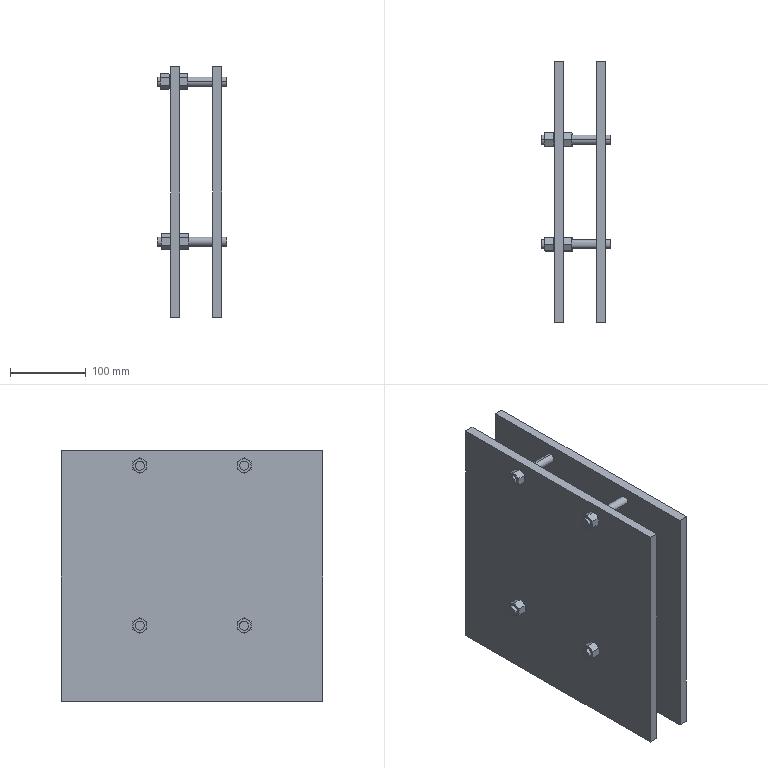Part | SolidWorks | 14 solids | 232 faces | box 90.963 x 344.147 x 330 mm | volume 2772183 mm3 | cone 108 | plane 84 | cylinder 40 | commonest cylinder face diameters 12 x40